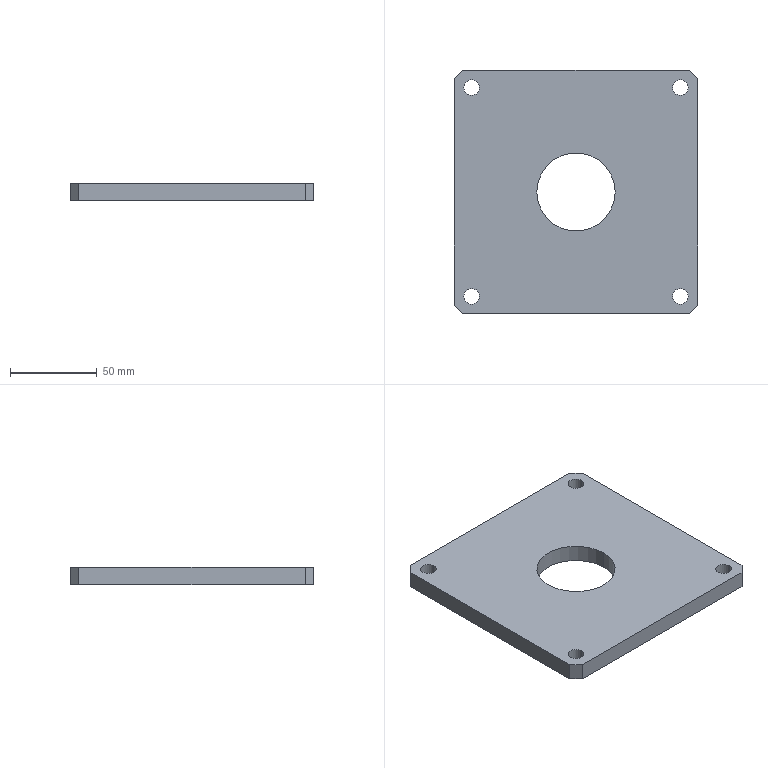Part | SolidWorks | features Chamfer 1, Extrusion 1, HoleWzd 1, ICE 1, LPattern 1 | 1 solid | 20 faces | box 140 x 140 x 10 mm | volume 177051 mm3 | cylinder 10 | plane 10 | commonest cylinder face diameters 9 x8 45 x2
STEP:
#1=CARTESIAN_POINT('',(22.5,0.,10.));
#2=VERTEX_POINT('',#1);
#3=CARTESIAN_POINT('',(-22.5,0.,10.));
#4=VERTEX_POINT('',#3);
#5=CARTESIAN_POINT('',(0.,0.,10.));
#6=DIRECTION('',(0.,0.,-1.));
#7=DIRECTION('',(-1.,0.,0.));
#8=AXIS2_PLACEMENT_3D('',#5,#6,#7);
#9=CIRCLE('',#8,22.5);
#10=EDGE_CURVE('',#2,#4,#9,.T.);
#11=ORIENTED_EDGE('',*,*,#10,.F.);
#12=CARTESIAN_POINT('',(22.5,0.,0.));
#13=VERTEX_POINT('',#12);
#14=CARTESIAN_POINT('',(22.5,0.,10.));
#15=DIRECTION('',(0.,0.,-1.));
#16=VECTOR('',#15,1000.);
#17=LINE('',#14,#16);
#18=EDGE_CURVE('',#2,#13,#17,.T.);
#19=ORIENTED_EDGE('',*,*,#18,.T.);
#20=CARTESIAN_POINT('',(-22.5,0.,0.));
#21=VERTEX_POINT('',#20);
#22=CARTESIAN_POINT('',(0.,0.,0.));
#23=DIRECTION('',(0.,0.,-1.));
#24=DIRECTION('',(-1.,0.,0.));
#25=AXIS2_PLACEMENT_3D('',#22,#23,#24);
#26=CIRCLE('',#25,22.5);
#27=EDGE_CURVE('',#13,#21,#26,.T.);
#28=ORIENTED_EDGE('',*,*,#27,.T.);
#29=CARTESIAN_POINT('',(-22.5,0.,10.));
#30=DIRECTION('',(0.,0.,-1.));
#31=VECTOR('',#30,1000.);
#32=LINE('',#29,#31);
#33=EDGE_CURVE('',#4,#21,#32,.T.);
#34=ORIENTED_EDGE('',*,*,#33,.F.);
#35=EDGE_LOOP('',(#11,#19,#28,#34));
#36=FACE_OUTER_BOUND('',#35,.T.);
#37=CARTESIAN_POINT('',(0.,0.,10.));
#38=DIRECTION('',(0.,0.,-1.));
#39=DIRECTION('',(-1.,0.,0.));
#40=AXIS2_PLACEMENT_3D('',#37,#38,#39);
#41=CYLINDRICAL_SURFACE('',#40,22.5);
#42=ADVANCED_FACE('',(#36),#41,.F.);
#43=CARTESIAN_POINT('',(64.5,60.,10.));
#44=VERTEX_POINT('',#43);
#45=CARTESIAN_POINT('',(55.5,60.,10.));
#46=VERTEX_POINT('',#45);
#47=CARTESIAN_POINT('',(60.,60.,10.));
#48=DIRECTION('',(0.,0.,-1.));
#49=DIRECTION('',(-1.,0.,0.));
#50=AXIS2_PLACEMENT_3D('',#47,#48,#49);
#51=CIRCLE('',#50,4.5);
#52=EDGE_CURVE('',#44,#46,#51,.T.);
#53=ORIENTED_EDGE('',*,*,#52,.F.);
#54=CARTESIAN_POINT('',(64.5,60.,0.));
#55=VERTEX_POINT('',#54);
#56=CARTESIAN_POINT('',(64.5,60.,0.));
#57=DIRECTION('',(0.,0.,-1.));
#58=VECTOR('',#57,1000.);
#59=LINE('',#56,#58);
#60=EDGE_CURVE('',#44,#55,#59,.T.);
#61=ORIENTED_EDGE('',*,*,#60,.T.);
#62=CARTESIAN_POINT('',(55.5,60.,0.));
#63=VERTEX_POINT('',#62);
#64=CARTESIAN_POINT('',(60.,60.,0.));
#65=DIRECTION('',(0.,0.,-1.));
#66=DIRECTION('',(-1.,0.,0.));
#67=AXIS2_PLACEMENT_3D('',#64,#65,#66);
#68=CIRCLE('',#67,4.5);
#69=EDGE_CURVE('',#55,#63,#68,.T.);
#70=ORIENTED_EDGE('',*,*,#69,.T.);
#71=CARTESIAN_POINT('',(55.5,60.,0.));
#72=DIRECTION('',(0.,0.,-1.));
#73=VECTOR('',#72,1000.);
#74=LINE('',#71,#73);
#75=EDGE_CURVE('',#46,#63,#74,.T.);
#76=ORIENTED_EDGE('',*,*,#75,.F.);
#77=EDGE_LOOP('',(#53,#61,#70,#76));
#78=FACE_OUTER_BOUND('',#77,.T.);
#79=CARTESIAN_POINT('',(60.,60.,0.));
#80=DIRECTION('',(0.,0.,-1.));
#81=DIRECTION('',(-1.,0.,0.));
#82=AXIS2_PLACEMENT_3D('',#79,#80,#81);
#83=CYLINDRICAL_SURFACE('',#82,4.5);
#84=ADVANCED_FACE('',(#78),#83,.F.);
#85=CARTESIAN_POINT('',(64.5,-60.,10.));
#86=VERTEX_POINT('',#85);
#87=CARTESIAN_POINT('',(55.5,-60.,10.));
#88=VERTEX_POINT('',#87);
#89=CARTESIAN_POINT('',(60.,-60.,10.));
#90=DIRECTION('',(0.,0.,-1.));
#91=DIRECTION('',(-1.,0.,0.));
#92=AXIS2_PLACEMENT_3D('',#89,#90,#91);
#93=CIRCLE('',#92,4.5);
#94=EDGE_CURVE('',#86,#88,#93,.T.);
#95=ORIENTED_EDGE('',*,*,#94,.F.);
#96=CARTESIAN_POINT('',(64.5,-60.,0.));
#97=VERTEX_POINT('',#96);
#98=CARTESIAN_POINT('',(64.5,-60.,0.));
#99=DIRECTION('',(0.,0.,-1.));
#100=VECTOR('',#99,1000.);
#101=LINE('',#98,#100);
#102=EDGE_CURVE('',#86,#97,#101,.T.);
#103=ORIENTED_EDGE('',*,*,#102,.T.);
#104=CARTESIAN_POINT('',(55.5,-60.,0.));
#105=VERTEX_POINT('',#104);
#106=CARTESIAN_POINT('',(60.,-60.,0.));
#107=DIRECTION('',(0.,0.,-1.));
#108=DIRECTION('',(-1.,0.,0.));
#109=AXIS2_PLACEMENT_3D('',#106,#107,#108);
#110=CIRCLE('',#109,4.5);
#111=EDGE_CURVE('',#97,#105,#110,.T.);
#112=ORIENTED_EDGE('',*,*,#111,.T.);
#113=CARTESIAN_POINT('',(55.5,-60.,0.));
#114=DIRECTION('',(0.,0.,-1.));
#115=VECTOR('',#114,1000.);
#116=LINE('',#113,#115);
#117=EDGE_CURVE('',#88,#105,#116,.T.);
#118=ORIENTED_EDGE('',*,*,#117,.F.);
#119=EDGE_LOOP('',(#95,#103,#112,#118));
#120=FACE_OUTER_BOUND('',#119,.T.);
#121=CARTESIAN_POINT('',(60.,-60.,0.));
#122=DIRECTION('',(0.,0.,-1.));
#123=DIRECTION('',(-1.,0.,0.));
#124=AXIS2_PLACEMENT_3D('',#121,#122,#123);
#125=CYLINDRICAL_SURFACE('',#124,4.5);
#126=ADVANCED_FACE('',(#120),#125,.F.);
#127=CARTESIAN_POINT('',(-55.5,-60.,10.));
#128=VERTEX_POINT('',#127);
#129=CARTESIAN_POINT('',(-64.5,-60.,10.));
#130=VERTEX_POINT('',#129);
#131=CARTESIAN_POINT('',(-60.,-60.,10.));
#132=DIRECTION('',(0.,0.,-1.));
#133=DIRECTION('',(-1.,0.,0.));
#134=AXIS2_PLACEMENT_3D('',#131,#132,#133);
#135=CIRCLE('',#134,4.5);
#136=EDGE_CURVE('',#128,#130,#135,.T.);
#137=ORIENTED_EDGE('',*,*,#136,.F.);
#138=CARTESIAN_POINT('',(-55.5,-60.,0.));
#139=VERTEX_POINT('',#138);
#140=CARTESIAN_POINT('',(-55.5,-60.,0.));
#141=DIRECTION('',(0.,0.,-1.));
#142=VECTOR('',#141,1000.);
#143=LINE('',#140,#142);
#144=EDGE_CURVE('',#128,#139,#143,.T.);
#145=ORIENTED_EDGE('',*,*,#144,.T.);
#146=CARTESIAN_POINT('',(-64.5,-60.,0.));
#147=VERTEX_POINT('',#146);
#148=CARTESIAN_POINT('',(-60.,-60.,0.));
#149=DIRECTION('',(0.,0.,-1.));
#150=DIRECTION('',(-1.,0.,0.));
#151=AXIS2_PLACEMENT_3D('',#148,#149,#150);
#152=CIRCLE('',#151,4.5);
#153=EDGE_CURVE('',#139,#147,#152,.T.);
#154=ORIENTED_EDGE('',*,*,#153,.T.);
#155=CARTESIAN_POINT('',(-64.5,-60.,0.));
#156=DIRECTION('',(0.,0.,-1.));
#157=VECTOR('',#156,1000.);
#158=LINE('',#155,#157);
#159=EDGE_CURVE('',#130,#147,#158,.T.);
#160=ORIENTED_EDGE('',*,*,#159,.F.);
#161=EDGE_LOOP('',(#137,#145,#154,#160));
#162=FACE_OUTER_BOUND('',#161,.T.);
#163=CARTESIAN_POINT('',(-60.,-60.,0.));
#164=DIRECTION('',(0.,0.,-1.));
#165=DIRECTION('',(-1.,0.,0.));
#166=AXIS2_PLACEMENT_3D('',#163,#164,#165);
#167=CYLINDRICAL_SURFACE('',#166,4.5);
#168=ADVANCED_FACE('',(#162),#167,.F.);
#169=CARTESIAN_POINT('',(-55.5,60.,10.));
#170=VERTEX_POINT('',#169);
#171=CARTESIAN_POINT('',(-64.5,60.,10.));
#172=VERTEX_POINT('',#171);
#173=CARTESIAN_POINT('',(-60.,60.,10.));
#174=DIRECTION('',(0.,0.,-1.));
#175=DIRECTION('',(-1.,0.,0.));
#176=AXIS2_PLACEMENT_3D('',#173,#174,#175);
#177=CIRCLE('',#176,4.5);
#178=EDGE_CURVE('',#170,#172,#177,.T.);
#179=ORIENTED_EDGE('',*,*,#178,.F.);
#180=CARTESIAN_POINT('',(-55.5,60.,0.));
#181=VERTEX_POINT('',#180);
#182=CARTESIAN_POINT('',(-55.5,60.,0.));
#183=DIRECTION('',(0.,0.,-1.));
#184=VECTOR('',#183,1000.);
#185=LINE('',#182,#184);
#186=EDGE_CURVE('',#170,#181,#185,.T.);
#187=ORIENTED_EDGE('',*,*,#186,.T.);
#188=CARTESIAN_POINT('',(-64.5,60.,0.));
#189=VERTEX_POINT('',#188);
#190=CARTESIAN_POINT('',(-60.,60.,0.));
#191=DIRECTION('',(0.,0.,-1.));
#192=DIRECTION('',(-1.,0.,0.));
#193=AXIS2_PLACEMENT_3D('',#190,#191,#192);
#194=CIRCLE('',#193,4.5);
#195=EDGE_CURVE('',#181,#189,#194,.T.);
#196=ORIENTED_EDGE('',*,*,#195,.T.);
#197=CARTESIAN_POINT('',(-64.5,60.,0.));
#198=DIRECTION('',(0.,0.,-1.));
#199=VECTOR('',#198,1000.);
#200=LINE('',#197,#199);
#201=EDGE_CURVE('',#172,#189,#200,.T.);
#202=ORIENTED_EDGE('',*,*,#201,.F.);
#203=EDGE_LOOP('',(#179,#187,#196,#202));
#204=FACE_OUTER_BOUND('',#203,.T.);
#205=CARTESIAN_POINT('',(-60.,60.,0.));
#206=DIRECTION('',(0.,0.,-1.));
#207=DIRECTION('',(-1.,0.,0.));
#208=AXIS2_PLACEMENT_3D('',#205,#206,#207);
#209=CYLINDRICAL_SURFACE('',#208,4.5);
#210=ADVANCED_FACE('',(#204),#209,.F.);
#211=ORIENTED_EDGE('',*,*,#186,.F.);
#212=CARTESIAN_POINT('',(-60.,60.,10.));
#213=DIRECTION('',(0.,0.,-1.));
#214=DIRECTION('',(-1.,0.,0.));
#215=AXIS2_PLACEMENT_3D('',#212,#213,#214);
#216=CIRCLE('',#215,4.5);
#217=EDGE_CURVE('',#172,#170,#216,.T.);
#218=ORIENTED_EDGE('',*,*,#217,.F.);
#219=ORIENTED_EDGE('',*,*,#201,.T.);
#220=CARTESIAN_POINT('',(-60.,60.,0.));
#221=DIRECTION('',(0.,0.,-1.));
#222=DIRECTION('',(-1.,0.,0.));
#223=AXIS2_PLACEMENT_3D('',#220,#221,#222);
#224=CIRCLE('',#223,4.5);
#225=EDGE_CURVE('',#189,#181,#224,.T.);
#226=ORIENTED_EDGE('',*,*,#225,.T.);
#227=EDGE_LOOP('',(#211,#218,#219,#226));
#228=FACE_OUTER_BOUND('',#227,.T.);
#229=CARTESIAN_POINT('',(-60.,60.,0.));
#230=DIRECTION('',(0.,0.,-1.));
#231=DIRECTION('',(-1.,0.,0.));
#232=AXIS2_PLACEMENT_3D('',#229,#230,#231);
#233=CYLINDRICAL_SURFACE('',#232,4.5);
#234=ADVANCED_FACE('',(#228),#233,.F.);
#235=ORIENTED_EDGE('',*,*,#144,.F.);
#236=CARTESIAN_POINT('',(-60.,-60.,10.));
#237=DIRECTION('',(0.,0.,-1.));
#238=DIRECTION('',(-1.,0.,0.));
#239=AXIS2_PLACEMENT_3D('',#236,#237,#238);
#240=CIRCLE('',#239,4.5);
#241=EDGE_CURVE('',#130,#128,#240,.T.);
#242=ORIENTED_EDGE('',*,*,#241,.F.);
#243=ORIENTED_EDGE('',*,*,#159,.T.);
#244=CARTESIAN_POINT('',(-60.,-60.,0.));
#245=DIRECTION('',(0.,0.,-1.));
#246=DIRECTION('',(-1.,0.,0.));
#247=AXIS2_PLACEMENT_3D('',#244,#245,#246);
#248=CIRCLE('',#247,4.5);
#249=EDGE_CURVE('',#147,#139,#248,.T.);
#250=ORIENTED_EDGE('',*,*,#249,.T.);
#251=EDGE_LOOP('',(#235,#242,#243,#250));
#252=FACE_OUTER_BOUND('',#251,.T.);
#253=CARTESIAN_POINT('',(-60.,-60.,0.));
#254=DIRECTION('',(0.,0.,-1.));
#255=DIRECTION('',(-1.,0.,0.));
#256=AXIS2_PLACEMENT_3D('',#253,#254,#255);
#257=CYLINDRICAL_SURFACE('',#256,4.5);
#258=ADVANCED_FACE('',(#252),#257,.F.);
#259=CARTESIAN_POINT('',(-70.,65.,10.));
#260=VERTEX_POINT('',#259);
#261=CARTESIAN_POINT('',(-70.,-65.,10.));
#262=VERTEX_POINT('',#261);
#263=CARTESIAN_POINT('',(-70.,70.,10.));
#264=DIRECTION('',(0.,-1.,0.));
#265=VECTOR('',#264,1000.);
#266=LINE('',#263,#265);
#267=EDGE_CURVE('',#260,#262,#266,.T.);
#268=ORIENTED_EDGE('',*,*,#267,.F.);
#269=CARTESIAN_POINT('',(-70.,65.,0.));
#270=VERTEX_POINT('',#269);
#271=CARTESIAN_POINT('',(-70.,65.,10.));
#272=DIRECTION('',(0.,0.,-1.));
#273=VECTOR('',#272,1000.);
#274=LINE('',#271,#273);
#275=EDGE_CURVE('',#260,#270,#274,.T.);
#276=ORIENTED_EDGE('',*,*,#275,.T.);
#277=CARTESIAN_POINT('',(-70.,-65.,0.));
#278=VERTEX_POINT('',#277);
#279=CARTESIAN_POINT('',(-70.,70.,0.));
#280=DIRECTION('',(0.,-1.,0.));
#281=VECTOR('',#280,1000.);
#282=LINE('',#279,#281);
#283=EDGE_CURVE('',#270,#278,#282,.T.);
#284=ORIENTED_EDGE('',*,*,#283,.T.);
#285=CARTESIAN_POINT('',(-70.,-65.,10.));
#286=DIRECTION('',(0.,0.,1.));
#287=VECTOR('',#286,1000.);
#288=LINE('',#285,#287);
#289=EDGE_CURVE('',#278,#262,#288,.T.);
#290=ORIENTED_EDGE('',*,*,#289,.T.);
#291=EDGE_LOOP('',(#268,#276,#284,#290));
#292=FACE_OUTER_BOUND('',#291,.T.);
#293=CARTESIAN_POINT('',(-70.,70.,10.));
#294=DIRECTION('',(1.,0.,0.));
#295=DIRECTION('',(0.,1.,0.));
#296=AXIS2_PLACEMENT_3D('',#293,#294,#295);
#297=PLANE('',#296);
#298=ADVANCED_FACE('',(#292),#297,.F.);
#299=CARTESIAN_POINT('',(-65.,-70.,0.));
#300=VERTEX_POINT('',#299);
#301=CARTESIAN_POINT('',(65.,-70.,0.));
#302=VERTEX_POINT('',#301);
#303=CARTESIAN_POINT('',(70.,-70.,0.));
#304=DIRECTION('',(1.,0.,0.));
#305=VECTOR('',#304,1000.);
#306=LINE('',#303,#305);
#307=EDGE_CURVE('',#300,#302,#306,.T.);
#308=ORIENTED_EDGE('',*,*,#307,.T.);
#309=CARTESIAN_POINT('',(65.,-70.,10.));
#310=VERTEX_POINT('',#309);
#311=CARTESIAN_POINT('',(65.,-70.,10.));
#312=DIRECTION('',(0.,0.,1.));
#313=VECTOR('',#312,1000.);
#314=LINE('',#311,#313);
#315=EDGE_CURVE('',#302,#310,#314,.T.);
#316=ORIENTED_EDGE('',*,*,#315,.T.);
#317=CARTESIAN_POINT('',(-65.,-70.,10.));
#318=VERTEX_POINT('',#317);
#319=CARTESIAN_POINT('',(70.,-70.,10.));
#320=DIRECTION('',(1.,0.,0.));
#321=VECTOR('',#320,1000.);
#322=LINE('',#319,#321);
#323=EDGE_CURVE('',#318,#310,#322,.T.);
#324=ORIENTED_EDGE('',*,*,#323,.F.);
#325=CARTESIAN_POINT('',(-65.,-70.,10.));
#326=DIRECTION('',(0.,0.,-1.));
#327=VECTOR('',#326,1000.);
#328=LINE('',#325,#327);
#329=EDGE_CURVE('',#318,#300,#328,.T.);
#330=ORIENTED_EDGE('',*,*,#329,.T.);
#331=EDGE_LOOP('',(#308,#316,#324,#330));
#332=FACE_OUTER_BOUND('',#331,.T.);
#333=CARTESIAN_POINT('',(70.,-70.,10.));
#334=DIRECTION('',(0.,1.,0.));
#335=DIRECTION('',(-1.,0.,0.));
#336=AXIS2_PLACEMENT_3D('',#333,#334,#335);
#337=PLANE('',#336);
#338=ADVANCED_FACE('',(#332),#337,.F.);
#339=CARTESIAN_POINT('',(70.,-65.,0.));
#340=VERTEX_POINT('',#339);
#341=CARTESIAN_POINT('',(70.,65.,0.));
#342=VERTEX_POINT('',#341);
#343=CARTESIAN_POINT('',(70.,70.,0.));
#344=DIRECTION('',(0.,1.,0.));
#345=VECTOR('',#344,1000.);
#346=LINE('',#343,#345);
#347=EDGE_CURVE('',#340,#342,#346,.T.);
#348=ORIENTED_EDGE('',*,*,#347,.T.);
#349=CARTESIAN_POINT('',(70.,65.,10.));
#350=VERTEX_POINT('',#349);
#351=CARTESIAN_POINT('',(70.,65.,10.));
#352=DIRECTION('',(0.,0.,1.));
#353=VECTOR('',#352,1000.);
#354=LINE('',#351,#353);
#355=EDGE_CURVE('',#342,#350,#354,.T.);
#356=ORIENTED_EDGE('',*,*,#355,.T.);
#357=CARTESIAN_POINT('',(70.,-65.,10.));
#358=VERTEX_POINT('',#357);
#359=CARTESIAN_POINT('',(70.,70.,10.));
#360=DIRECTION('',(0.,1.,0.));
#361=VECTOR('',#360,1000.);
#362=LINE('',#359,#361);
#363=EDGE_CURVE('',#358,#350,#362,.T.);
#364=ORIENTED_EDGE('',*,*,#363,.F.);
#365=CARTESIAN_POINT('',(70.,-65.,10.));
#366=DIRECTION('',(0.,0.,-1.));
#367=VECTOR('',#366,1000.);
#368=LINE('',#365,#367);
#369=EDGE_CURVE('',#358,#340,#368,.T.);
#370=ORIENTED_EDGE('',*,*,#369,.T.);
#371=EDGE_LOOP('',(#348,#356,#364,#370));
#372=FACE_OUTER_BOUND('',#371,.T.);
#373=CARTESIAN_POINT('',(70.,70.,10.));
#374=DIRECTION('',(-1.,0.,0.));
#375=DIRECTION('',(0.,-1.,0.));
#376=AXIS2_PLACEMENT_3D('',#373,#374,#375);
#377=PLANE('',#376);
#378=ADVANCED_FACE('',(#372),#377,.F.);
#379=CARTESIAN_POINT('',(65.,70.,0.));
#380=VERTEX_POINT('',#379);
#381=CARTESIAN_POINT('',(-65.,70.,0.));
#382=VERTEX_POINT('',#381);
#383=CARTESIAN_POINT('',(70.,70.,0.));
#384=DIRECTION('',(-1.,0.,0.));
#385=VECTOR('',#384,1000.);
#386=LINE('',#383,#385);
#387=EDGE_CURVE('',#380,#382,#386,.T.);
#388=ORIENTED_EDGE('',*,*,#387,.T.);
#389=CARTESIAN_POINT('',(-65.,70.,10.));
#390=VERTEX_POINT('',#389);
#391=CARTESIAN_POINT('',(-65.,70.,10.));
#392=DIRECTION('',(0.,0.,1.));
#393=VECTOR('',#392,1000.);
#394=LINE('',#391,#393);
#395=EDGE_CURVE('',#382,#390,#394,.T.);
#396=ORIENTED_EDGE('',*,*,#395,.T.);
#397=CARTESIAN_POINT('',(65.,70.,10.));
#398=VERTEX_POINT('',#397);
#399=CARTESIAN_POINT('',(70.,70.,10.));
#400=DIRECTION('',(-1.,0.,0.));
#401=VECTOR('',#400,1000.);
#402=LINE('',#399,#401);
#403=EDGE_CURVE('',#398,#390,#402,.T.);
#404=ORIENTED_EDGE('',*,*,#403,.F.);
#405=CARTESIAN_POINT('',(65.,70.,10.));
#406=DIRECTION('',(0.,0.,-1.));
#407=VECTOR('',#406,1000.);
#408=LINE('',#405,#407);
#409=EDGE_CURVE('',#398,#380,#408,.T.);
#410=ORIENTED_EDGE('',*,*,#409,.T.);
#411=EDGE_LOOP('',(#388,#396,#404,#410));
#412=FACE_OUTER_BOUND('',#411,.T.);
#413=CARTESIAN_POINT('',(70.,70.,10.));
#414=DIRECTION('',(0.,-1.,0.));
#415=DIRECTION('',(1.,0.,0.));
#416=AXIS2_PLACEMENT_3D('',#413,#414,#415);
#417=PLANE('',#416);
#418=ADVANCED_FACE('',(#412),#417,.F.);
#419=CARTESIAN_POINT('',(0.,0.,10.));
#420=DIRECTION('',(0.,0.,-1.));
#421=DIRECTION('',(-1.,0.,0.));
#422=AXIS2_PLACEMENT_3D('',#419,#420,#421);
#423=CIRCLE('',#422,22.5);
#424=EDGE_CURVE('',#4,#2,#423,.T.);
#425=ORIENTED_EDGE('',*,*,#424,.T.);
#426=ORIENTED_EDGE('',*,*,#10,.T.);
#427=EDGE_LOOP('',(#425,#426));
#428=FACE_BOUND('',#427,.T.);
#429=CARTESIAN_POINT('',(60.,60.,10.));
#430=DIRECTION('',(0.,0.,-1.));
#431=DIRECTION('',(-1.,0.,0.));
#432=AXIS2_PLACEMENT_3D('',#429,#430,#431);
#433=CIRCLE('',#432,4.5);
#434=EDGE_CURVE('',#46,#44,#433,.T.);
#435=ORIENTED_EDGE('',*,*,#434,.T.);
#436=ORIENTED_EDGE('',*,*,#52,.T.);
#437=EDGE_LOOP('',(#435,#436));
#438=FACE_BOUND('',#437,.T.);
#439=CARTESIAN_POINT('',(60.,-60.,10.));
#440=DIRECTION('',(0.,0.,-1.));
#441=DIRECTION('',(-1.,0.,0.));
#442=AXIS2_PLACEMENT_3D('',#439,#440,#441);
#443=CIRCLE('',#442,4.5);
#444=EDGE_CURVE('',#88,#86,#443,.T.);
#445=ORIENTED_EDGE('',*,*,#444,.T.);
#446=ORIENTED_EDGE('',*,*,#94,.T.);
#447=EDGE_LOOP('',(#445,#446));
#448=FACE_BOUND('',#447,.T.);
#449=ORIENTED_EDGE('',*,*,#403,.T.);
#450=CARTESIAN_POINT('',(-70.,65.,10.));
#451=DIRECTION('',(-0.7071,-0.7071,0.));
#452=VECTOR('',#451,1000.);
#453=LINE('',#450,#452);
#454=EDGE_CURVE('',#390,#260,#453,.T.);
#455=ORIENTED_EDGE('',*,*,#454,.T.);
#456=ORIENTED_EDGE('',*,*,#267,.T.);
#457=CARTESIAN_POINT('',(-65.,-70.,10.));
#458=DIRECTION('',(0.7071,-0.7071,0.));
#459=VECTOR('',#458,1000.);
#460=LINE('',#457,#459);
#461=EDGE_CURVE('',#262,#318,#460,.T.);
#462=ORIENTED_EDGE('',*,*,#461,.T.);
#463=ORIENTED_EDGE('',*,*,#323,.T.);
#464=CARTESIAN_POINT('',(70.,-65.,10.));
#465=DIRECTION('',(0.7071,0.7071,0.));
#466=VECTOR('',#465,1000.);
#467=LINE('',#464,#466);
#468=EDGE_CURVE('',#310,#358,#467,.T.);
#469=ORIENTED_EDGE('',*,*,#468,.T.);
#470=ORIENTED_EDGE('',*,*,#363,.T.);
#471=CARTESIAN_POINT('',(65.,70.,10.));
#472=DIRECTION('',(-0.7071,0.7071,0.));
#473=VECTOR('',#472,1000.);
#474=LINE('',#471,#473);
#475=EDGE_CURVE('',#350,#398,#474,.T.);
#476=ORIENTED_EDGE('',*,*,#475,.T.);
#477=EDGE_LOOP('',(#449,#455,#456,#462,#463,#469,#470,#476));
#478=FACE_OUTER_BOUND('',#477,.T.);
#479=ORIENTED_EDGE('',*,*,#241,.T.);
#480=ORIENTED_EDGE('',*,*,#136,.T.);
#481=EDGE_LOOP('',(#479,#480));
#482=FACE_BOUND('',#481,.T.);
#483=ORIENTED_EDGE('',*,*,#217,.T.);
#484=ORIENTED_EDGE('',*,*,#178,.T.);
#485=EDGE_LOOP('',(#483,#484));
#486=FACE_BOUND('',#485,.T.);
#487=CARTESIAN_POINT('',(0.,0.,10.));
#488=DIRECTION('',(0.,0.,-1.));
#489=DIRECTION('',(-1.,0.,0.));
#490=AXIS2_PLACEMENT_3D('',#487,#488,#489);
#491=PLANE('',#490);
#492=ADVANCED_FACE('',(#428,#438,#448,#478,#482,#486),#491,.F.);
#493=CARTESIAN_POINT('',(0.,0.,0.));
#494=DIRECTION('',(0.,0.,-1.));
#495=DIRECTION('',(-1.,0.,0.));
#496=AXIS2_PLACEMENT_3D('',#493,#494,#495);
#497=CIRCLE('',#496,22.5);
#498=EDGE_CURVE('',#21,#13,#497,.T.);
#499=ORIENTED_EDGE('',*,*,#498,.F.);
#500=ORIENTED_EDGE('',*,*,#27,.F.);
#501=EDGE_LOOP('',(#499,#500));
#502=FACE_BOUND('',#501,.T.);
#503=CARTESIAN_POINT('',(60.,60.,0.));
#504=DIRECTION('',(0.,0.,-1.));
#505=DIRECTION('',(-1.,0.,0.));
#506=AXIS2_PLACEMENT_3D('',#503,#504,#505);
#507=CIRCLE('',#506,4.5);
#508=EDGE_CURVE('',#63,#55,#507,.T.);
#509=ORIENTED_EDGE('',*,*,#508,.F.);
#510=ORIENTED_EDGE('',*,*,#69,.F.);
#511=EDGE_LOOP('',(#509,#510));
#512=FACE_BOUND('',#511,.T.);
#513=CARTESIAN_POINT('',(60.,-60.,0.));
#514=DIRECTION('',(0.,0.,-1.));
#515=DIRECTION('',(-1.,0.,0.));
#516=AXIS2_PLACEMENT_3D('',#513,#514,#515);
#517=CIRCLE('',#516,4.5);
#518=EDGE_CURVE('',#105,#97,#517,.T.);
#519=ORIENTED_EDGE('',*,*,#518,.F.);
#520=ORIENTED_EDGE('',*,*,#111,.F.);
#521=EDGE_LOOP('',(#519,#520));
#522=FACE_BOUND('',#521,.T.);
#523=ORIENTED_EDGE('',*,*,#283,.F.);
#524=CARTESIAN_POINT('',(-67.5,67.5,0.));
#525=DIRECTION('',(0.7071,0.7071,0.));
#526=VECTOR('',#525,1000.);
#527=LINE('',#524,#526);
#528=EDGE_CURVE('',#270,#382,#527,.T.);
#529=ORIENTED_EDGE('',*,*,#528,.T.);
#530=ORIENTED_EDGE('',*,*,#387,.F.);
#531=CARTESIAN_POINT('',(67.5,67.5,0.));
#532=DIRECTION('',(0.7071,-0.7071,0.));
#533=VECTOR('',#532,1000.);
#534=LINE('',#531,#533);
#535=EDGE_CURVE('',#380,#342,#534,.T.);
#536=ORIENTED_EDGE('',*,*,#535,.T.);
#537=ORIENTED_EDGE('',*,*,#347,.F.);
#538=CARTESIAN_POINT('',(67.5,-67.5,0.));
#539=DIRECTION('',(-0.7071,-0.7071,0.));
#540=VECTOR('',#539,1000.);
#541=LINE('',#538,#540);
#542=EDGE_CURVE('',#340,#302,#541,.T.);
#543=ORIENTED_EDGE('',*,*,#542,.T.);
#544=ORIENTED_EDGE('',*,*,#307,.F.);
#545=CARTESIAN_POINT('',(-67.5,-67.5,0.));
#546=DIRECTION('',(-0.7071,0.7071,0.));
#547=VECTOR('',#546,1000.);
#548=LINE('',#545,#547);
#549=EDGE_CURVE('',#300,#278,#548,.T.);
#550=ORIENTED_EDGE('',*,*,#549,.T.);
#551=EDGE_LOOP('',(#523,#529,#530,#536,#537,#543,#544,#550));
#552=FACE_OUTER_BOUND('',#551,.T.);
#553=ORIENTED_EDGE('',*,*,#249,.F.);
#554=ORIENTED_EDGE('',*,*,#153,.F.);
#555=EDGE_LOOP('',(#553,#554));
#556=FACE_BOUND('',#555,.T.);
#557=ORIENTED_EDGE('',*,*,#225,.F.);
#558=ORIENTED_EDGE('',*,*,#195,.F.);
#559=EDGE_LOOP('',(#557,#558));
#560=FACE_BOUND('',#559,.T.);
#561=CARTESIAN_POINT('',(0.,0.,0.));
#562=DIRECTION('',(0.,0.,-1.));
#563=DIRECTION('',(-1.,0.,0.));
#564=AXIS2_PLACEMENT_3D('',#561,#562,#563);
#565=PLANE('',#564);
#566=ADVANCED_FACE('',(#502,#512,#522,#552,#556,#560),#565,.T.);
#567=ORIENTED_EDGE('',*,*,#454,.F.);
#568=ORIENTED_EDGE('',*,*,#395,.F.);
#569=ORIENTED_EDGE('',*,*,#528,.F.);
#570=ORIENTED_EDGE('',*,*,#275,.F.);
#571=EDGE_LOOP('',(#567,#568,#569,#570));
#572=FACE_OUTER_BOUND('',#571,.T.);
#573=CARTESIAN_POINT('',(-70.,65.,10.));
#574=DIRECTION('',(0.7071,-0.7071,0.));
#575=DIRECTION('',(0.,0.,-1.));
#576=AXIS2_PLACEMENT_3D('',#573,#574,#575);
#577=PLANE('',#576);
#578=ADVANCED_FACE('',(#572),#577,.F.);
#579=ORIENTED_EDGE('',*,*,#475,.F.);
#580=ORIENTED_EDGE('',*,*,#355,.F.);
#581=ORIENTED_EDGE('',*,*,#535,.F.);
#582=ORIENTED_EDGE('',*,*,#409,.F.);
#583=EDGE_LOOP('',(#579,#580,#581,#582));
#584=FACE_OUTER_BOUND('',#583,.T.);
#585=CARTESIAN_POINT('',(65.,70.,10.));
#586=DIRECTION('',(-0.7071,-0.7071,0.));
#587=DIRECTION('',(0.,0.,-1.));
#588=AXIS2_PLACEMENT_3D('',#585,#586,#587);
#589=PLANE('',#588);
#590=ADVANCED_FACE('',(#584),#589,.F.);
#591=ORIENTED_EDGE('',*,*,#468,.F.);
#592=ORIENTED_EDGE('',*,*,#315,.F.);
#593=ORIENTED_EDGE('',*,*,#542,.F.);
#594=ORIENTED_EDGE('',*,*,#369,.F.);
#595=EDGE_LOOP('',(#591,#592,#593,#594));
#596=FACE_OUTER_BOUND('',#595,.T.);
#597=CARTESIAN_POINT('',(70.,-65.,10.));
#598=DIRECTION('',(-0.7071,0.7071,0.));
#599=DIRECTION('',(0.,0.,-1.));
#600=AXIS2_PLACEMENT_3D('',#597,#598,#599);
#601=PLANE('',#600);
#602=ADVANCED_FACE('',(#596),#601,.F.);
#603=ORIENTED_EDGE('',*,*,#461,.F.);
#604=ORIENTED_EDGE('',*,*,#289,.F.);
#605=ORIENTED_EDGE('',*,*,#549,.F.);
#606=ORIENTED_EDGE('',*,*,#329,.F.);
#607=EDGE_LOOP('',(#603,#604,#605,#606));
#608=FACE_OUTER_BOUND('',#607,.T.);
#609=CARTESIAN_POINT('',(-65.,-70.,10.));
#610=DIRECTION('',(0.7071,0.7071,0.));
#611=DIRECTION('',(0.,0.,-1.));
#612=AXIS2_PLACEMENT_3D('',#609,#610,#611);
#613=PLANE('',#612);
#614=ADVANCED_FACE('',(#608),#613,.F.);
#615=ORIENTED_EDGE('',*,*,#102,.F.);
#616=ORIENTED_EDGE('',*,*,#444,.F.);
#617=ORIENTED_EDGE('',*,*,#117,.T.);
#618=ORIENTED_EDGE('',*,*,#518,.T.);
#619=EDGE_LOOP('',(#615,#616,#617,#618));
#620=FACE_OUTER_BOUND('',#619,.T.);
#621=CARTESIAN_POINT('',(60.,-60.,0.));
#622=DIRECTION('',(0.,0.,-1.));
#623=DIRECTION('',(-1.,0.,0.));
#624=AXIS2_PLACEMENT_3D('',#621,#622,#623);
#625=CYLINDRICAL_SURFACE('',#624,4.5);
#626=ADVANCED_FACE('',(#620),#625,.F.);
#627=ORIENTED_EDGE('',*,*,#60,.F.);
#628=ORIENTED_EDGE('',*,*,#434,.F.);
#629=ORIENTED_EDGE('',*,*,#75,.T.);
#630=ORIENTED_EDGE('',*,*,#508,.T.);
#631=EDGE_LOOP('',(#627,#628,#629,#630));
#632=FACE_OUTER_BOUND('',#631,.T.);
#633=CARTESIAN_POINT('',(60.,60.,0.));
#634=DIRECTION('',(0.,0.,-1.));
#635=DIRECTION('',(-1.,0.,0.));
#636=AXIS2_PLACEMENT_3D('',#633,#634,#635);
#637=CYLINDRICAL_SURFACE('',#636,4.5);
#638=ADVANCED_FACE('',(#632),#637,.F.);
#639=ORIENTED_EDGE('',*,*,#18,.F.);
#640=ORIENTED_EDGE('',*,*,#424,.F.);
#641=ORIENTED_EDGE('',*,*,#33,.T.);
#642=ORIENTED_EDGE('',*,*,#498,.T.);
#643=EDGE_LOOP('',(#639,#640,#641,#642));
#644=FACE_OUTER_BOUND('',#643,.T.);
#645=CARTESIAN_POINT('',(0.,0.,10.));
#646=DIRECTION('',(0.,0.,-1.));
#647=DIRECTION('',(-1.,0.,0.));
#648=AXIS2_PLACEMENT_3D('',#645,#646,#647);
#649=CYLINDRICAL_SURFACE('',#648,22.5);
#650=ADVANCED_FACE('',(#644),#649,.F.);
#651=CLOSED_SHELL('',(#42,#84,#126,#168,#210,#234,#258,#298,#338,#378,#418,#492,#566,#578,#590,#602,#614,#626,#638,#650));
#652=MANIFOLD_SOLID_BREP('',#651);
#653=CARTESIAN_POINT('',(0.,0.,0.));
#654=DIRECTION('',(0.,0.,1.));
#655=DIRECTION('',(1.,0.,0.));
#656=AXIS2_PLACEMENT_3D('',#653,#654,#655);
#657=(LENGTH_UNIT()NAMED_UNIT(*)SI_UNIT(.MILLI.,.METRE.));
#658=UNCERTAINTY_MEASURE_WITH_UNIT(LENGTH_MEASURE(0.00001),#657,'','');
#659=(NAMED_UNIT(*)PLANE_ANGLE_UNIT()SI_UNIT($,.RADIAN.));
#660=(NAMED_UNIT(*)SI_UNIT($,.STERADIAN.)SOLID_ANGLE_UNIT());
#661=(GEOMETRIC_REPRESENTATION_CONTEXT(3)GLOBAL_UNCERTAINTY_ASSIGNED_CONTEXT((#658))GLOBAL_UNIT_ASSIGNED_CONTEXT((#657,#659,#660))REPRESENTATION_CONTEXT('',''));
#662=ADVANCED_BREP_SHAPE_REPRESENTATION('',(#652,#656),#661);